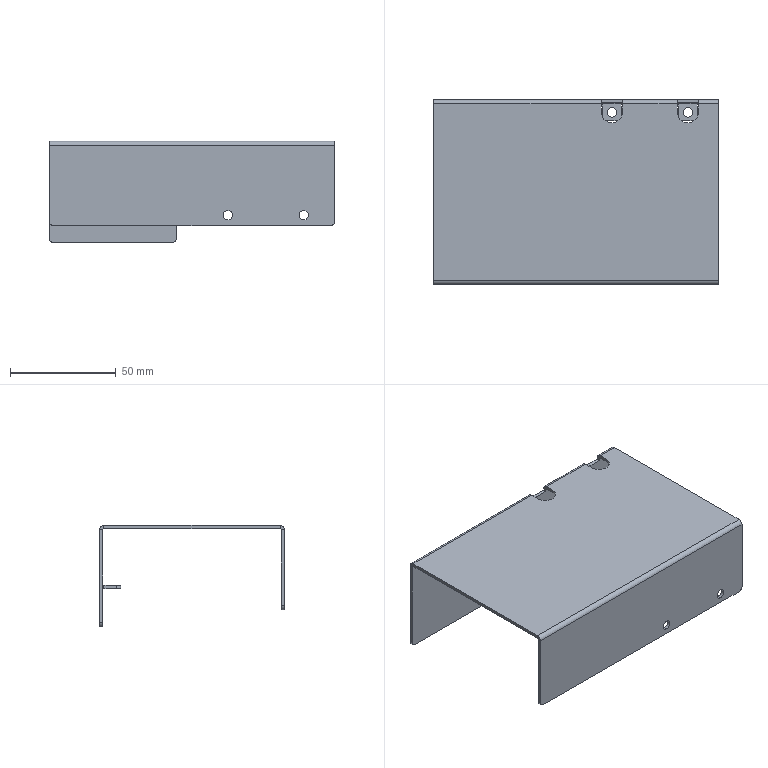Part | STEP file | Belt guard | 1 solid | 85 faces | box 135 x 87.5 x 48 mm | volume 32458 mm3 | plane 54 | cylinder 31 | commonest cylinder face diameters 4 x15 4.5 x8 1 x6 10 x2